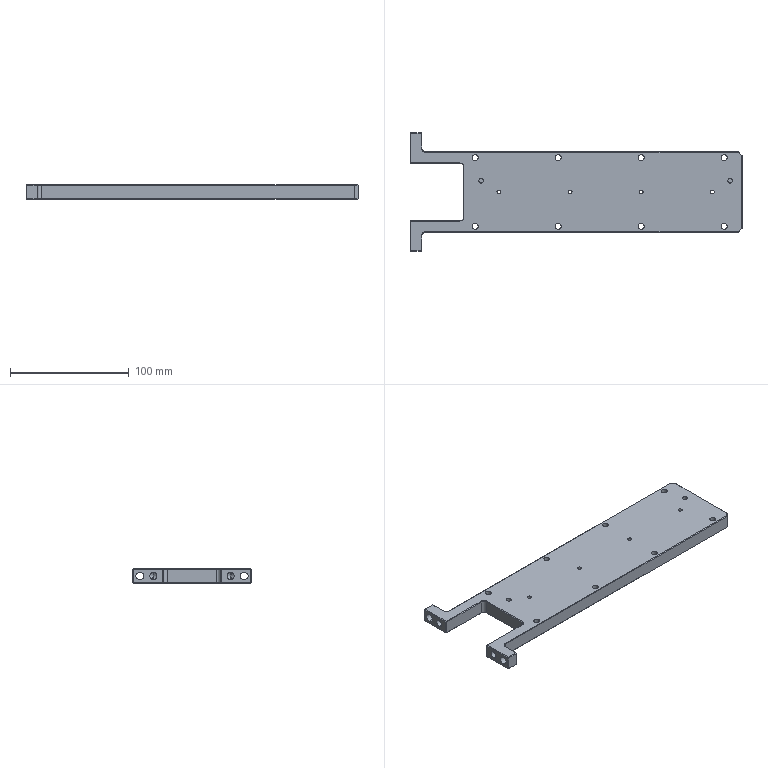Part | SolidWorks | features HoleWzd 7, Chamfer 2, Fillet 2, Cut 1, Extrusion 1, ICE 1 | 1 solid | 132 faces | box 280 x 100 x 12 mm | volume 201479 mm3 | plane 64 | cylinder 48 | cone 20 | commonest cylinder face diameters 5 x20 6 x12 3.3 x8 4 x4 6.6 x4